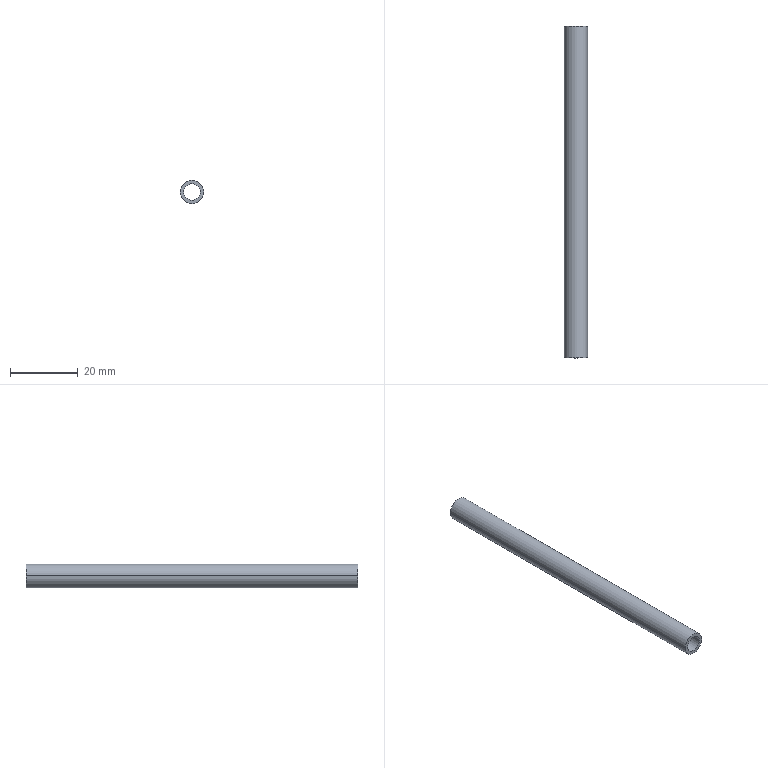Part | SolidWorks | features BaseBody 1 | 1 solid | 6 faces | box 6.9 x 97.77 x 6.9 mm | volume 1812 mm3 | cylinder 4 | plane 2 | commonest cylinder face diameters 4.9 x2 6.9 x2
STEP:
#1=CARTESIAN_POINT('',(-47.55,-120.,0.));
#2=VERTEX_POINT('',#1);
#3=CARTESIAN_POINT('',(-52.45,-120.,0.));
#4=VERTEX_POINT('',#3);
#5=CARTESIAN_POINT('',(-50.,-120.,0.));
#6=DIRECTION('',(0.,-1.,0.));
#7=DIRECTION('',(1.,0.,0.));
#8=AXIS2_PLACEMENT_3D('',#5,#6,#7);
#9=CIRCLE('',#8,2.45);
#10=EDGE_CURVE('',#2,#4,#9,.T.);
#11=ORIENTED_EDGE('',*,*,#10,.F.);
#12=CARTESIAN_POINT('',(-50.,-120.,0.));
#13=DIRECTION('',(0.,-1.,0.));
#14=DIRECTION('',(-1.,0.,0.));
#15=AXIS2_PLACEMENT_3D('',#12,#13,#14);
#16=CIRCLE('',#15,2.45);
#17=EDGE_CURVE('',#4,#2,#16,.T.);
#18=ORIENTED_EDGE('',*,*,#17,.F.);
#19=EDGE_LOOP('',(#11,#18));
#20=FACE_BOUND('',#19,.T.);
#21=CARTESIAN_POINT('',(-46.55,-120.,0.));
#22=VERTEX_POINT('',#21);
#23=CARTESIAN_POINT('',(-53.45,-120.,0.));
#24=VERTEX_POINT('',#23);
#25=CARTESIAN_POINT('',(-50.,-120.,0.));
#26=DIRECTION('',(0.,1.,0.));
#27=DIRECTION('',(1.,0.,0.));
#28=AXIS2_PLACEMENT_3D('',#25,#26,#27);
#29=CIRCLE('',#28,3.45);
#30=EDGE_CURVE('',#22,#24,#29,.T.);
#31=ORIENTED_EDGE('',*,*,#30,.F.);
#32=CARTESIAN_POINT('',(-50.,-120.,0.));
#33=DIRECTION('',(0.,1.,0.));
#34=DIRECTION('',(-1.,0.,0.));
#35=AXIS2_PLACEMENT_3D('',#32,#33,#34);
#36=CIRCLE('',#35,3.45);
#37=EDGE_CURVE('',#24,#22,#36,.T.);
#38=ORIENTED_EDGE('',*,*,#37,.F.);
#39=EDGE_LOOP('',(#31,#38));
#40=FACE_OUTER_BOUND('',#39,.T.);
#41=CARTESIAN_POINT('',(-50.,-120.,0.));
#42=DIRECTION('',(0.,-1.,0.));
#43=DIRECTION('',(0.,0.,-1.));
#44=AXIS2_PLACEMENT_3D('',#41,#42,#43);
#45=PLANE('',#44);
#46=ADVANCED_FACE('',(#20,#40),#45,.T.);
#47=CARTESIAN_POINT('',(-47.55,-22.23,0.));
#48=VERTEX_POINT('',#47);
#49=CARTESIAN_POINT('',(-52.45,-22.23,0.));
#50=VERTEX_POINT('',#49);
#51=CARTESIAN_POINT('',(-50.,-22.23,0.));
#52=DIRECTION('',(0.,1.,0.));
#53=DIRECTION('',(1.,0.,0.));
#54=AXIS2_PLACEMENT_3D('',#51,#52,#53);
#55=CIRCLE('',#54,2.45);
#56=EDGE_CURVE('',#48,#50,#55,.T.);
#57=ORIENTED_EDGE('',*,*,#56,.F.);
#58=CARTESIAN_POINT('',(-50.,-22.23,0.));
#59=DIRECTION('',(0.,1.,0.));
#60=DIRECTION('',(-1.,0.,0.));
#61=AXIS2_PLACEMENT_3D('',#58,#59,#60);
#62=CIRCLE('',#61,2.45);
#63=EDGE_CURVE('',#50,#48,#62,.T.);
#64=ORIENTED_EDGE('',*,*,#63,.F.);
#65=EDGE_LOOP('',(#57,#64));
#66=FACE_BOUND('',#65,.T.);
#67=CARTESIAN_POINT('',(-46.55,-22.23,0.));
#68=VERTEX_POINT('',#67);
#69=CARTESIAN_POINT('',(-53.45,-22.23,0.));
#70=VERTEX_POINT('',#69);
#71=CARTESIAN_POINT('',(-50.,-22.23,0.));
#72=DIRECTION('',(0.,-1.,0.));
#73=DIRECTION('',(1.,0.,0.));
#74=AXIS2_PLACEMENT_3D('',#71,#72,#73);
#75=CIRCLE('',#74,3.45);
#76=EDGE_CURVE('',#68,#70,#75,.T.);
#77=ORIENTED_EDGE('',*,*,#76,.F.);
#78=CARTESIAN_POINT('',(-50.,-22.23,0.));
#79=DIRECTION('',(0.,-1.,0.));
#80=DIRECTION('',(-1.,0.,0.));
#81=AXIS2_PLACEMENT_3D('',#78,#79,#80);
#82=CIRCLE('',#81,3.45);
#83=EDGE_CURVE('',#70,#68,#82,.T.);
#84=ORIENTED_EDGE('',*,*,#83,.F.);
#85=EDGE_LOOP('',(#77,#84));
#86=FACE_OUTER_BOUND('',#85,.T.);
#87=CARTESIAN_POINT('',(-50.,-22.23,0.));
#88=DIRECTION('',(0.,1.,0.));
#89=DIRECTION('',(1.,0.,0.));
#90=AXIS2_PLACEMENT_3D('',#87,#88,#89);
#91=PLANE('',#90);
#92=ADVANCED_FACE('',(#66,#86),#91,.T.);
#93=ORIENTED_EDGE('',*,*,#37,.T.);
#94=CARTESIAN_POINT('',(-46.55,-22.23,0.));
#95=DIRECTION('',(0.,-1.,0.));
#96=VECTOR('',#95,1000.);
#97=LINE('',#94,#96);
#98=EDGE_CURVE('',#68,#22,#97,.T.);
#99=ORIENTED_EDGE('',*,*,#98,.F.);
#100=ORIENTED_EDGE('',*,*,#76,.T.);
#101=CARTESIAN_POINT('',(-53.45,-120.,0.));
#102=DIRECTION('',(0.,1.,0.));
#103=VECTOR('',#102,1000.);
#104=LINE('',#101,#103);
#105=EDGE_CURVE('',#24,#70,#104,.T.);
#106=ORIENTED_EDGE('',*,*,#105,.F.);
#107=EDGE_LOOP('',(#93,#99,#100,#106));
#108=FACE_OUTER_BOUND('',#107,.T.);
#109=CARTESIAN_POINT('',(-50.,-22.23,0.));
#110=DIRECTION('',(0.,-1.,0.));
#111=DIRECTION('',(1.,0.,0.));
#112=AXIS2_PLACEMENT_3D('',#109,#110,#111);
#113=CYLINDRICAL_SURFACE('',#112,3.45);
#114=ADVANCED_FACE('',(#108),#113,.T.);
#115=ORIENTED_EDGE('',*,*,#105,.T.);
#116=ORIENTED_EDGE('',*,*,#83,.T.);
#117=ORIENTED_EDGE('',*,*,#98,.T.);
#118=ORIENTED_EDGE('',*,*,#30,.T.);
#119=EDGE_LOOP('',(#115,#116,#117,#118));
#120=FACE_OUTER_BOUND('',#119,.T.);
#121=CARTESIAN_POINT('',(-50.,-22.23,0.));
#122=DIRECTION('',(0.,-1.,0.));
#123=DIRECTION('',(1.,0.,0.));
#124=AXIS2_PLACEMENT_3D('',#121,#122,#123);
#125=CYLINDRICAL_SURFACE('',#124,3.45);
#126=ADVANCED_FACE('',(#120),#125,.T.);
#127=ORIENTED_EDGE('',*,*,#17,.T.);
#128=CARTESIAN_POINT('',(-47.55,-22.23,0.));
#129=DIRECTION('',(0.,-1.,0.));
#130=VECTOR('',#129,1000.);
#131=LINE('',#128,#130);
#132=EDGE_CURVE('',#48,#2,#131,.T.);
#133=ORIENTED_EDGE('',*,*,#132,.F.);
#134=ORIENTED_EDGE('',*,*,#56,.T.);
#135=CARTESIAN_POINT('',(-52.45,-120.,0.));
#136=DIRECTION('',(0.,1.,0.));
#137=VECTOR('',#136,1000.);
#138=LINE('',#135,#137);
#139=EDGE_CURVE('',#4,#50,#138,.T.);
#140=ORIENTED_EDGE('',*,*,#139,.F.);
#141=EDGE_LOOP('',(#127,#133,#134,#140));
#142=FACE_OUTER_BOUND('',#141,.T.);
#143=CARTESIAN_POINT('',(-50.,-22.23,0.));
#144=DIRECTION('',(0.,-1.,0.));
#145=DIRECTION('',(1.,0.,0.));
#146=AXIS2_PLACEMENT_3D('',#143,#144,#145);
#147=CYLINDRICAL_SURFACE('',#146,2.45);
#148=ADVANCED_FACE('',(#142),#147,.F.);
#149=ORIENTED_EDGE('',*,*,#139,.T.);
#150=ORIENTED_EDGE('',*,*,#63,.T.);
#151=ORIENTED_EDGE('',*,*,#132,.T.);
#152=ORIENTED_EDGE('',*,*,#10,.T.);
#153=EDGE_LOOP('',(#149,#150,#151,#152));
#154=FACE_OUTER_BOUND('',#153,.T.);
#155=CARTESIAN_POINT('',(-50.,-22.23,0.));
#156=DIRECTION('',(0.,-1.,0.));
#157=DIRECTION('',(1.,0.,0.));
#158=AXIS2_PLACEMENT_3D('',#155,#156,#157);
#159=CYLINDRICAL_SURFACE('',#158,2.45);
#160=ADVANCED_FACE('',(#154),#159,.F.);
#161=CLOSED_SHELL('',(#46,#92,#114,#126,#148,#160));
#162=MANIFOLD_SOLID_BREP('',#161);
#163=CARTESIAN_POINT('',(0.,0.,0.));
#164=DIRECTION('',(0.,0.,1.));
#165=DIRECTION('',(1.,0.,0.));
#166=AXIS2_PLACEMENT_3D('',#163,#164,#165);
#167=(LENGTH_UNIT()NAMED_UNIT(*)SI_UNIT(.MILLI.,.METRE.));
#168=UNCERTAINTY_MEASURE_WITH_UNIT(LENGTH_MEASURE(0.00001),#167,'','');
#169=(NAMED_UNIT(*)PLANE_ANGLE_UNIT()SI_UNIT($,.RADIAN.));
#170=(NAMED_UNIT(*)SI_UNIT($,.STERADIAN.)SOLID_ANGLE_UNIT());
#171=(GEOMETRIC_REPRESENTATION_CONTEXT(3)GLOBAL_UNCERTAINTY_ASSIGNED_CONTEXT((#168))GLOBAL_UNIT_ASSIGNED_CONTEXT((#167,#169,#170))REPRESENTATION_CONTEXT('',''));
#172=ADVANCED_BREP_SHAPE_REPRESENTATION('',(#162,#166),#171);